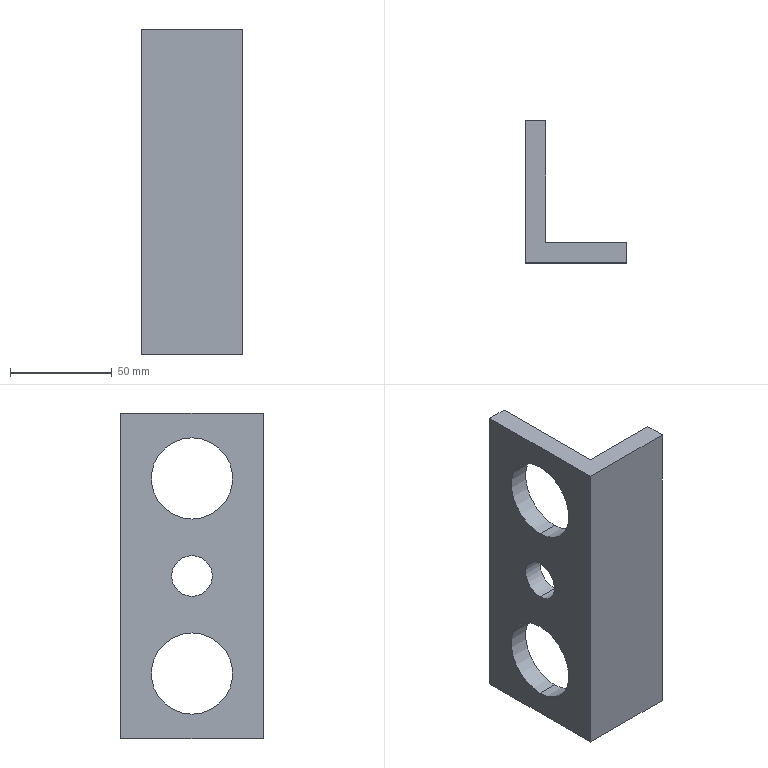Part | STEP file | 1 solid | 14 faces | box 50 x 70 x 160 mm | volume 147726 mm3 | plane 8 | cylinder 6 | commonest cylinder face diameters 40 x4 20 x2
STEP:
#1=CARTESIAN_POINT('',(0.,0.,0.));
#2=DIRECTION('',(0.,0.,1.));
#3=DIRECTION('',(1.,0.,0.));
#4=AXIS2_PLACEMENT_3D('',#1,#2,#3);
#5=CARTESIAN_POINT('',(-10.,25.,-10.));
#6=VERTEX_POINT('',#5);
#7=CARTESIAN_POINT('',(0.,25.,-10.));
#8=VERTEX_POINT('',#7);
#9=CARTESIAN_POINT('',(13.,25.,-10.));
#10=DIRECTION('',(1.,0.,0.));
#11=VECTOR('',#10,1.);
#12=LINE('',#9,#11);
#13=CARTESIAN_POINT('',(13.,25.,0.));
#14=DIRECTION('',(1.,0.,0.));
#15=DIRECTION('',(0.,0.,-1.));
#16=AXIS2_PLACEMENT_3D('',#13,#14,#15);
#17=CYLINDRICAL_SURFACE('',#16,10.);
#18=CARTESIAN_POINT('',(6.283,0.));
#19=DIRECTION('',(0.,1.));
#20=VECTOR('',#19,1.);
#21=LINE('',#18,#20);
#22=(GEOMETRIC_REPRESENTATION_CONTEXT(2)PARAMETRIC_REPRESENTATION_CONTEXT()REPRESENTATION_CONTEXT('',''));
#23=DEFINITIONAL_REPRESENTATION('',(#21),#22);
#24=PCURVE('',#17,#23);
#25=CARTESIAN_POINT('',(13.,25.,0.));
#26=DIRECTION('',(1.,0.,0.));
#27=DIRECTION('',(0.,0.,-1.));
#28=AXIS2_PLACEMENT_3D('',#25,#26,#27);
#29=CYLINDRICAL_SURFACE('',#28,10.);
#30=CARTESIAN_POINT('',(0.,0.));
#31=DIRECTION('',(0.,1.));
#32=VECTOR('',#31,1.);
#33=LINE('',#30,#32);
#34=(GEOMETRIC_REPRESENTATION_CONTEXT(2)PARAMETRIC_REPRESENTATION_CONTEXT()REPRESENTATION_CONTEXT('',''));
#35=DEFINITIONAL_REPRESENTATION('',(#33),#34);
#36=PCURVE('',#29,#35);
#37=SURFACE_CURVE('',#12,(#24,#36),.PCURVE_S1.);
#38=EDGE_CURVE('',#6,#8,#37,.T.);
#39=ORIENTED_EDGE('',*,*,#38,.T.);
#40=CARTESIAN_POINT('',(0.,25.,10.));
#41=VERTEX_POINT('',#40);
#42=CARTESIAN_POINT('',(0.,25.,0.));
#43=DIRECTION('',(-1.,0.,0.));
#44=DIRECTION('',(0.,0.,-1.));
#45=AXIS2_PLACEMENT_3D('',#42,#43,#44);
#46=CIRCLE('',#45,10.);
#47=CARTESIAN_POINT('',(6.283,-13.));
#48=DIRECTION('',(-1.,0.));
#49=VECTOR('',#48,1.);
#50=LINE('',#47,#49);
#51=(GEOMETRIC_REPRESENTATION_CONTEXT(2)PARAMETRIC_REPRESENTATION_CONTEXT()REPRESENTATION_CONTEXT('',''));
#52=DEFINITIONAL_REPRESENTATION('',(#50),#51);
#53=PCURVE('',#17,#52);
#54=CARTESIAN_POINT('',(0.,60.,80.));
#55=DIRECTION('',(1.,0.,0.));
#56=DIRECTION('',(0.,1.,0.));
#57=AXIS2_PLACEMENT_3D('',#54,#55,#56);
#58=PLANE('',#57);
#59=CARTESIAN_POINT('',(-35.,-90.));
#60=CARTESIAN_POINT('',(-52.321,-90.));
#61=CARTESIAN_POINT('',(-43.66,-75.));
#62=CARTESIAN_POINT('',(-35.,-60.));
#63=CARTESIAN_POINT('',(-26.34,-75.));
#64=CARTESIAN_POINT('',(-17.679,-90.));
#65=CARTESIAN_POINT('',(-35.,-90.));
#66=(BOUNDED_CURVE()B_SPLINE_CURVE(2,(#59,#60,#61,#62,#63,#64,#65),.UNSPECIFIED.,.T.,.F.)B_SPLINE_CURVE_WITH_KNOTS((1,2,2,2,2,1),(-2.094,0.,2.094,4.189,6.283,8.378),.UNSPECIFIED.)CURVE()GEOMETRIC_REPRESENTATION_ITEM()RATIONAL_B_SPLINE_CURVE((1.,0.5,1.,0.5,1.,0.5,1.))REPRESENTATION_ITEM(''));
#67=(GEOMETRIC_REPRESENTATION_CONTEXT(2)PARAMETRIC_REPRESENTATION_CONTEXT()REPRESENTATION_CONTEXT('',''));
#68=DEFINITIONAL_REPRESENTATION('',(#66),#67);
#69=PCURVE('',#58,#68);
#70=SURFACE_CURVE('',#46,(#53,#69),.PCURVE_S1.);
#71=EDGE_CURVE('',#8,#41,#70,.T.);
#72=ORIENTED_EDGE('',*,*,#71,.T.);
#73=CARTESIAN_POINT('',(-10.,25.,10.));
#74=VERTEX_POINT('',#73);
#75=CARTESIAN_POINT('',(13.,25.,10.));
#76=DIRECTION('',(1.,0.,0.));
#77=VECTOR('',#76,1.);
#78=LINE('',#75,#77);
#79=CARTESIAN_POINT('',(3.142,0.));
#80=DIRECTION('',(0.,1.));
#81=VECTOR('',#80,1.);
#82=LINE('',#79,#81);
#83=(GEOMETRIC_REPRESENTATION_CONTEXT(2)PARAMETRIC_REPRESENTATION_CONTEXT()REPRESENTATION_CONTEXT('',''));
#84=DEFINITIONAL_REPRESENTATION('',(#82),#83);
#85=PCURVE('',#17,#84);
#86=CARTESIAN_POINT('',(3.142,0.));
#87=DIRECTION('',(0.,1.));
#88=VECTOR('',#87,1.);
#89=LINE('',#86,#88);
#90=(GEOMETRIC_REPRESENTATION_CONTEXT(2)PARAMETRIC_REPRESENTATION_CONTEXT()REPRESENTATION_CONTEXT('',''));
#91=DEFINITIONAL_REPRESENTATION('',(#89),#90);
#92=PCURVE('',#29,#91);
#93=SURFACE_CURVE('',#78,(#85,#92),.PCURVE_S1.);
#94=EDGE_CURVE('',#74,#41,#93,.T.);
#95=ORIENTED_EDGE('',*,*,#94,.F.);
#96=CARTESIAN_POINT('',(-10.,25.,0.));
#97=DIRECTION('',(-1.,0.,0.));
#98=DIRECTION('',(0.,0.,-1.));
#99=AXIS2_PLACEMENT_3D('',#96,#97,#98);
#100=CIRCLE('',#99,10.);
#101=CARTESIAN_POINT('',(6.283,-23.));
#102=DIRECTION('',(-1.,0.));
#103=VECTOR('',#102,1.);
#104=LINE('',#101,#103);
#105=(GEOMETRIC_REPRESENTATION_CONTEXT(2)PARAMETRIC_REPRESENTATION_CONTEXT()REPRESENTATION_CONTEXT('',''));
#106=DEFINITIONAL_REPRESENTATION('',(#104),#105);
#107=PCURVE('',#17,#106);
#108=CARTESIAN_POINT('',(-10.,60.,80.));
#109=DIRECTION('',(1.,0.,0.));
#110=DIRECTION('',(0.,1.,0.));
#111=AXIS2_PLACEMENT_3D('',#108,#109,#110);
#112=PLANE('',#111);
#113=CARTESIAN_POINT('',(-35.,-90.));
#114=CARTESIAN_POINT('',(-52.321,-90.));
#115=CARTESIAN_POINT('',(-43.66,-75.));
#116=CARTESIAN_POINT('',(-35.,-60.));
#117=CARTESIAN_POINT('',(-26.34,-75.));
#118=CARTESIAN_POINT('',(-17.679,-90.));
#119=CARTESIAN_POINT('',(-35.,-90.));
#120=(BOUNDED_CURVE()B_SPLINE_CURVE(2,(#113,#114,#115,#116,#117,#118,#119),.UNSPECIFIED.,.T.,.F.)B_SPLINE_CURVE_WITH_KNOTS((1,2,2,2,2,1),(-2.094,0.,2.094,4.189,6.283,8.378),.UNSPECIFIED.)CURVE()GEOMETRIC_REPRESENTATION_ITEM()RATIONAL_B_SPLINE_CURVE((1.,0.5,1.,0.5,1.,0.5,1.))REPRESENTATION_ITEM(''));
#121=(GEOMETRIC_REPRESENTATION_CONTEXT(2)PARAMETRIC_REPRESENTATION_CONTEXT()REPRESENTATION_CONTEXT('',''));
#122=DEFINITIONAL_REPRESENTATION('',(#120),#121);
#123=PCURVE('',#112,#122);
#124=SURFACE_CURVE('',#100,(#107,#123),.PCURVE_S1.);
#125=EDGE_CURVE('',#6,#74,#124,.T.);
#126=ORIENTED_EDGE('',*,*,#125,.F.);
#127=EDGE_LOOP('',(#39,#72,#95,#126));
#128=FACE_BOUND('',#127,.F.);
#129=ADVANCED_FACE('',(#128),#17,.F.);
#130=CARTESIAN_POINT('',(-10.,25.,28.));
#131=VERTEX_POINT('',#130);
#132=CARTESIAN_POINT('',(0.,25.,28.));
#133=VERTEX_POINT('',#132);
#134=CARTESIAN_POINT('',(13.,25.,28.));
#135=DIRECTION('',(1.,0.,0.));
#136=VECTOR('',#135,1.);
#137=LINE('',#134,#136);
#138=CARTESIAN_POINT('',(13.,25.,48.));
#139=DIRECTION('',(1.,0.,0.));
#140=DIRECTION('',(0.,0.,-1.));
#141=AXIS2_PLACEMENT_3D('',#138,#139,#140);
#142=CYLINDRICAL_SURFACE('',#141,20.);
#143=CARTESIAN_POINT('',(6.283,0.));
#144=DIRECTION('',(0.,1.));
#145=VECTOR('',#144,1.);
#146=LINE('',#143,#145);
#147=(GEOMETRIC_REPRESENTATION_CONTEXT(2)PARAMETRIC_REPRESENTATION_CONTEXT()REPRESENTATION_CONTEXT('',''));
#148=DEFINITIONAL_REPRESENTATION('',(#146),#147);
#149=PCURVE('',#142,#148);
#150=CARTESIAN_POINT('',(13.,25.,48.));
#151=DIRECTION('',(1.,0.,0.));
#152=DIRECTION('',(0.,0.,-1.));
#153=AXIS2_PLACEMENT_3D('',#150,#151,#152);
#154=CYLINDRICAL_SURFACE('',#153,20.);
#155=CARTESIAN_POINT('',(0.,0.));
#156=DIRECTION('',(0.,1.));
#157=VECTOR('',#156,1.);
#158=LINE('',#155,#157);
#159=(GEOMETRIC_REPRESENTATION_CONTEXT(2)PARAMETRIC_REPRESENTATION_CONTEXT()REPRESENTATION_CONTEXT('',''));
#160=DEFINITIONAL_REPRESENTATION('',(#158),#159);
#161=PCURVE('',#154,#160);
#162=SURFACE_CURVE('',#137,(#149,#161),.PCURVE_S1.);
#163=EDGE_CURVE('',#131,#133,#162,.T.);
#164=ORIENTED_EDGE('',*,*,#163,.T.);
#165=CARTESIAN_POINT('',(0.,25.,68.));
#166=VERTEX_POINT('',#165);
#167=CARTESIAN_POINT('',(0.,25.,48.));
#168=DIRECTION('',(-1.,0.,0.));
#169=DIRECTION('',(0.,0.,-1.));
#170=AXIS2_PLACEMENT_3D('',#167,#168,#169);
#171=CIRCLE('',#170,20.);
#172=CARTESIAN_POINT('',(6.283,-13.));
#173=DIRECTION('',(-1.,0.));
#174=VECTOR('',#173,1.);
#175=LINE('',#172,#174);
#176=(GEOMETRIC_REPRESENTATION_CONTEXT(2)PARAMETRIC_REPRESENTATION_CONTEXT()REPRESENTATION_CONTEXT('',''));
#177=DEFINITIONAL_REPRESENTATION('',(#175),#176);
#178=PCURVE('',#142,#177);
#179=CARTESIAN_POINT('',(-35.,-52.));
#180=CARTESIAN_POINT('',(-69.641,-52.));
#181=CARTESIAN_POINT('',(-52.321,-22.));
#182=CARTESIAN_POINT('',(-35.,8.));
#183=CARTESIAN_POINT('',(-17.679,-22.));
#184=CARTESIAN_POINT('',(-0.359,-52.));
#185=CARTESIAN_POINT('',(-35.,-52.));
#186=(BOUNDED_CURVE()B_SPLINE_CURVE(2,(#179,#180,#181,#182,#183,#184,#185),.UNSPECIFIED.,.T.,.F.)B_SPLINE_CURVE_WITH_KNOTS((1,2,2,2,2,1),(-2.094,0.,2.094,4.189,6.283,8.378),.UNSPECIFIED.)CURVE()GEOMETRIC_REPRESENTATION_ITEM()RATIONAL_B_SPLINE_CURVE((1.,0.5,1.,0.5,1.,0.5,1.))REPRESENTATION_ITEM(''));
#187=(GEOMETRIC_REPRESENTATION_CONTEXT(2)PARAMETRIC_REPRESENTATION_CONTEXT()REPRESENTATION_CONTEXT('',''));
#188=DEFINITIONAL_REPRESENTATION('',(#186),#187);
#189=PCURVE('',#58,#188);
#190=SURFACE_CURVE('',#171,(#178,#189),.PCURVE_S1.);
#191=EDGE_CURVE('',#133,#166,#190,.T.);
#192=ORIENTED_EDGE('',*,*,#191,.T.);
#193=CARTESIAN_POINT('',(-10.,25.,68.));
#194=VERTEX_POINT('',#193);
#195=CARTESIAN_POINT('',(13.,25.,68.));
#196=DIRECTION('',(1.,0.,0.));
#197=VECTOR('',#196,1.);
#198=LINE('',#195,#197);
#199=CARTESIAN_POINT('',(3.142,0.));
#200=DIRECTION('',(0.,1.));
#201=VECTOR('',#200,1.);
#202=LINE('',#199,#201);
#203=(GEOMETRIC_REPRESENTATION_CONTEXT(2)PARAMETRIC_REPRESENTATION_CONTEXT()REPRESENTATION_CONTEXT('',''));
#204=DEFINITIONAL_REPRESENTATION('',(#202),#203);
#205=PCURVE('',#142,#204);
#206=CARTESIAN_POINT('',(3.142,0.));
#207=DIRECTION('',(0.,1.));
#208=VECTOR('',#207,1.);
#209=LINE('',#206,#208);
#210=(GEOMETRIC_REPRESENTATION_CONTEXT(2)PARAMETRIC_REPRESENTATION_CONTEXT()REPRESENTATION_CONTEXT('',''));
#211=DEFINITIONAL_REPRESENTATION('',(#209),#210);
#212=PCURVE('',#154,#211);
#213=SURFACE_CURVE('',#198,(#205,#212),.PCURVE_S1.);
#214=EDGE_CURVE('',#194,#166,#213,.T.);
#215=ORIENTED_EDGE('',*,*,#214,.F.);
#216=CARTESIAN_POINT('',(-10.,25.,48.));
#217=DIRECTION('',(-1.,0.,0.));
#218=DIRECTION('',(0.,0.,-1.));
#219=AXIS2_PLACEMENT_3D('',#216,#217,#218);
#220=CIRCLE('',#219,20.);
#221=CARTESIAN_POINT('',(6.283,-23.));
#222=DIRECTION('',(-1.,0.));
#223=VECTOR('',#222,1.);
#224=LINE('',#221,#223);
#225=(GEOMETRIC_REPRESENTATION_CONTEXT(2)PARAMETRIC_REPRESENTATION_CONTEXT()REPRESENTATION_CONTEXT('',''));
#226=DEFINITIONAL_REPRESENTATION('',(#224),#225);
#227=PCURVE('',#142,#226);
#228=CARTESIAN_POINT('',(-35.,-52.));
#229=CARTESIAN_POINT('',(-69.641,-52.));
#230=CARTESIAN_POINT('',(-52.321,-22.));
#231=CARTESIAN_POINT('',(-35.,8.));
#232=CARTESIAN_POINT('',(-17.679,-22.));
#233=CARTESIAN_POINT('',(-0.359,-52.));
#234=CARTESIAN_POINT('',(-35.,-52.));
#235=(BOUNDED_CURVE()B_SPLINE_CURVE(2,(#228,#229,#230,#231,#232,#233,#234),.UNSPECIFIED.,.T.,.F.)B_SPLINE_CURVE_WITH_KNOTS((1,2,2,2,2,1),(-2.094,0.,2.094,4.189,6.283,8.378),.UNSPECIFIED.)CURVE()GEOMETRIC_REPRESENTATION_ITEM()RATIONAL_B_SPLINE_CURVE((1.,0.5,1.,0.5,1.,0.5,1.))REPRESENTATION_ITEM(''));
#236=(GEOMETRIC_REPRESENTATION_CONTEXT(2)PARAMETRIC_REPRESENTATION_CONTEXT()REPRESENTATION_CONTEXT('',''));
#237=DEFINITIONAL_REPRESENTATION('',(#235),#236);
#238=PCURVE('',#112,#237);
#239=SURFACE_CURVE('',#220,(#227,#238),.PCURVE_S1.);
#240=EDGE_CURVE('',#131,#194,#239,.T.);
#241=ORIENTED_EDGE('',*,*,#240,.F.);
#242=EDGE_LOOP('',(#164,#192,#215,#241));
#243=FACE_BOUND('',#242,.F.);
#244=ADVANCED_FACE('',(#243),#142,.F.);
#245=CARTESIAN_POINT('',(-10.,25.,-68.));
#246=VERTEX_POINT('',#245);
#247=CARTESIAN_POINT('',(0.,25.,-68.));
#248=VERTEX_POINT('',#247);
#249=CARTESIAN_POINT('',(13.,25.,-68.));
#250=DIRECTION('',(1.,0.,0.));
#251=VECTOR('',#250,1.);
#252=LINE('',#249,#251);
#253=CARTESIAN_POINT('',(13.,25.,-48.));
#254=DIRECTION('',(1.,0.,0.));
#255=DIRECTION('',(0.,0.,-1.));
#256=AXIS2_PLACEMENT_3D('',#253,#254,#255);
#257=CYLINDRICAL_SURFACE('',#256,20.);
#258=CARTESIAN_POINT('',(6.283,0.));
#259=DIRECTION('',(0.,1.));
#260=VECTOR('',#259,1.);
#261=LINE('',#258,#260);
#262=(GEOMETRIC_REPRESENTATION_CONTEXT(2)PARAMETRIC_REPRESENTATION_CONTEXT()REPRESENTATION_CONTEXT('',''));
#263=DEFINITIONAL_REPRESENTATION('',(#261),#262);
#264=PCURVE('',#257,#263);
#265=CARTESIAN_POINT('',(13.,25.,-48.));
#266=DIRECTION('',(1.,0.,0.));
#267=DIRECTION('',(0.,0.,-1.));
#268=AXIS2_PLACEMENT_3D('',#265,#266,#267);
#269=CYLINDRICAL_SURFACE('',#268,20.);
#270=CARTESIAN_POINT('',(0.,0.));
#271=DIRECTION('',(0.,1.));
#272=VECTOR('',#271,1.);
#273=LINE('',#270,#272);
#274=(GEOMETRIC_REPRESENTATION_CONTEXT(2)PARAMETRIC_REPRESENTATION_CONTEXT()REPRESENTATION_CONTEXT('',''));
#275=DEFINITIONAL_REPRESENTATION('',(#273),#274);
#276=PCURVE('',#269,#275);
#277=SURFACE_CURVE('',#252,(#264,#276),.PCURVE_S1.);
#278=EDGE_CURVE('',#246,#248,#277,.T.);
#279=ORIENTED_EDGE('',*,*,#278,.T.);
#280=CARTESIAN_POINT('',(0.,25.,-28.));
#281=VERTEX_POINT('',#280);
#282=CARTESIAN_POINT('',(0.,25.,-48.));
#283=DIRECTION('',(-1.,0.,0.));
#284=DIRECTION('',(0.,0.,-1.));
#285=AXIS2_PLACEMENT_3D('',#282,#283,#284);
#286=CIRCLE('',#285,20.);
#287=CARTESIAN_POINT('',(6.283,-13.));
#288=DIRECTION('',(-1.,0.));
#289=VECTOR('',#288,1.);
#290=LINE('',#287,#289);
#291=(GEOMETRIC_REPRESENTATION_CONTEXT(2)PARAMETRIC_REPRESENTATION_CONTEXT()REPRESENTATION_CONTEXT('',''));
#292=DEFINITIONAL_REPRESENTATION('',(#290),#291);
#293=PCURVE('',#257,#292);
#294=CARTESIAN_POINT('',(-35.,-148.));
#295=CARTESIAN_POINT('',(-69.641,-148.));
#296=CARTESIAN_POINT('',(-52.321,-118.));
#297=CARTESIAN_POINT('',(-35.,-88.));
#298=CARTESIAN_POINT('',(-17.679,-118.));
#299=CARTESIAN_POINT('',(-0.359,-148.));
#300=CARTESIAN_POINT('',(-35.,-148.));
#301=(BOUNDED_CURVE()B_SPLINE_CURVE(2,(#294,#295,#296,#297,#298,#299,#300),.UNSPECIFIED.,.T.,.F.)B_SPLINE_CURVE_WITH_KNOTS((1,2,2,2,2,1),(-2.094,0.,2.094,4.189,6.283,8.378),.UNSPECIFIED.)CURVE()GEOMETRIC_REPRESENTATION_ITEM()RATIONAL_B_SPLINE_CURVE((1.,0.5,1.,0.5,1.,0.5,1.))REPRESENTATION_ITEM(''));
#302=(GEOMETRIC_REPRESENTATION_CONTEXT(2)PARAMETRIC_REPRESENTATION_CONTEXT()REPRESENTATION_CONTEXT('',''));
#303=DEFINITIONAL_REPRESENTATION('',(#301),#302);
#304=PCURVE('',#58,#303);
#305=SURFACE_CURVE('',#286,(#293,#304),.PCURVE_S1.);
#306=EDGE_CURVE('',#248,#281,#305,.T.);
#307=ORIENTED_EDGE('',*,*,#306,.T.);
#308=CARTESIAN_POINT('',(-10.,25.,-28.));
#309=VERTEX_POINT('',#308);
#310=CARTESIAN_POINT('',(13.,25.,-28.));
#311=DIRECTION('',(1.,0.,0.));
#312=VECTOR('',#311,1.);
#313=LINE('',#310,#312);
#314=CARTESIAN_POINT('',(3.142,0.));
#315=DIRECTION('',(0.,1.));
#316=VECTOR('',#315,1.);
#317=LINE('',#314,#316);
#318=(GEOMETRIC_REPRESENTATION_CONTEXT(2)PARAMETRIC_REPRESENTATION_CONTEXT()REPRESENTATION_CONTEXT('',''));
#319=DEFINITIONAL_REPRESENTATION('',(#317),#318);
#320=PCURVE('',#257,#319);
#321=CARTESIAN_POINT('',(3.142,0.));
#322=DIRECTION('',(0.,1.));
#323=VECTOR('',#322,1.);
#324=LINE('',#321,#323);
#325=(GEOMETRIC_REPRESENTATION_CONTEXT(2)PARAMETRIC_REPRESENTATION_CONTEXT()REPRESENTATION_CONTEXT('',''));
#326=DEFINITIONAL_REPRESENTATION('',(#324),#325);
#327=PCURVE('',#269,#326);
#328=SURFACE_CURVE('',#313,(#320,#327),.PCURVE_S1.);
#329=EDGE_CURVE('',#309,#281,#328,.T.);
#330=ORIENTED_EDGE('',*,*,#329,.F.);
#331=CARTESIAN_POINT('',(-10.,25.,-48.));
#332=DIRECTION('',(-1.,0.,0.));
#333=DIRECTION('',(0.,0.,-1.));
#334=AXIS2_PLACEMENT_3D('',#331,#332,#333);
#335=CIRCLE('',#334,20.);
#336=CARTESIAN_POINT('',(6.283,-23.));
#337=DIRECTION('',(-1.,0.));
#338=VECTOR('',#337,1.);
#339=LINE('',#336,#338);
#340=(GEOMETRIC_REPRESENTATION_CONTEXT(2)PARAMETRIC_REPRESENTATION_CONTEXT()REPRESENTATION_CONTEXT('',''));
#341=DEFINITIONAL_REPRESENTATION('',(#339),#340);
#342=PCURVE('',#257,#341);
#343=CARTESIAN_POINT('',(-35.,-148.));
#344=CARTESIAN_POINT('',(-69.641,-148.));
#345=CARTESIAN_POINT('',(-52.321,-118.));
#346=CARTESIAN_POINT('',(-35.,-88.));
#347=CARTESIAN_POINT('',(-17.679,-118.));
#348=CARTESIAN_POINT('',(-0.359,-148.));
#349=CARTESIAN_POINT('',(-35.,-148.));
#350=(BOUNDED_CURVE()B_SPLINE_CURVE(2,(#343,#344,#345,#346,#347,#348,#349),.UNSPECIFIED.,.T.,.F.)B_SPLINE_CURVE_WITH_KNOTS((1,2,2,2,2,1),(-2.094,0.,2.094,4.189,6.283,8.378),.UNSPECIFIED.)CURVE()GEOMETRIC_REPRESENTATION_ITEM()RATIONAL_B_SPLINE_CURVE((1.,0.5,1.,0.5,1.,0.5,1.))REPRESENTATION_ITEM(''));
#351=(GEOMETRIC_REPRESENTATION_CONTEXT(2)PARAMETRIC_REPRESENTATION_CONTEXT()REPRESENTATION_CONTEXT('',''));
#352=DEFINITIONAL_REPRESENTATION('',(#350),#351);
#353=PCURVE('',#112,#352);
#354=SURFACE_CURVE('',#335,(#342,#353),.PCURVE_S1.);
#355=EDGE_CURVE('',#246,#309,#354,.T.);
#356=ORIENTED_EDGE('',*,*,#355,.F.);
#357=EDGE_LOOP('',(#279,#307,#330,#356));
#358=FACE_BOUND('',#357,.F.);
#359=ADVANCED_FACE('',(#358),#257,.F.);
#360=ORIENTED_EDGE('',*,*,#125,.F.);
#361=CARTESIAN_POINT('',(-10.,25.,0.));
#362=DIRECTION('',(-1.,0.,0.));
#363=DIRECTION('',(0.,0.,-1.));
#364=AXIS2_PLACEMENT_3D('',#361,#362,#363);
#365=CIRCLE('',#364,10.);
#366=CARTESIAN_POINT('',(-35.,-90.));
#367=CARTESIAN_POINT('',(-52.321,-90.));
#368=CARTESIAN_POINT('',(-43.66,-75.));
#369=CARTESIAN_POINT('',(-35.,-60.));
#370=CARTESIAN_POINT('',(-26.34,-75.));
#371=CARTESIAN_POINT('',(-17.679,-90.));
#372=CARTESIAN_POINT('',(-35.,-90.));
#373=(BOUNDED_CURVE()B_SPLINE_CURVE(2,(#366,#367,#368,#369,#370,#371,#372),.UNSPECIFIED.,.T.,.F.)B_SPLINE_CURVE_WITH_KNOTS((1,2,2,2,2,1),(-2.094,0.,2.094,4.189,6.283,8.378),.UNSPECIFIED.)CURVE()GEOMETRIC_REPRESENTATION_ITEM()RATIONAL_B_SPLINE_CURVE((1.,0.5,1.,0.5,1.,0.5,1.))REPRESENTATION_ITEM(''));
#374=(GEOMETRIC_REPRESENTATION_CONTEXT(2)PARAMETRIC_REPRESENTATION_CONTEXT()REPRESENTATION_CONTEXT('',''));
#375=DEFINITIONAL_REPRESENTATION('',(#373),#374);
#376=PCURVE('',#112,#375);
#377=CARTESIAN_POINT('',(6.283,-23.));
#378=DIRECTION('',(-1.,0.));
#379=VECTOR('',#378,1.);
#380=LINE('',#377,#379);
#381=(GEOMETRIC_REPRESENTATION_CONTEXT(2)PARAMETRIC_REPRESENTATION_CONTEXT()REPRESENTATION_CONTEXT('',''));
#382=DEFINITIONAL_REPRESENTATION('',(#380),#381);
#383=PCURVE('',#29,#382);
#384=SURFACE_CURVE('',#365,(#376,#383),.PCURVE_S1.);
#385=EDGE_CURVE('',#74,#6,#384,.T.);
#386=ORIENTED_EDGE('',*,*,#385,.F.);
#387=EDGE_LOOP('',(#360,#386));
#388=FACE_BOUND('',#387,.T.);
#389=ORIENTED_EDGE('',*,*,#240,.F.);
#390=CARTESIAN_POINT('',(-10.,25.,48.));
#391=DIRECTION('',(-1.,0.,0.));
#392=DIRECTION('',(0.,0.,-1.));
#393=AXIS2_PLACEMENT_3D('',#390,#391,#392);
#394=CIRCLE('',#393,20.);
#395=CARTESIAN_POINT('',(-35.,-52.));
#396=CARTESIAN_POINT('',(-69.641,-52.));
#397=CARTESIAN_POINT('',(-52.321,-22.));
#398=CARTESIAN_POINT('',(-35.,8.));
#399=CARTESIAN_POINT('',(-17.679,-22.));
#400=CARTESIAN_POINT('',(-0.359,-52.));
#401=CARTESIAN_POINT('',(-35.,-52.));
#402=(BOUNDED_CURVE()B_SPLINE_CURVE(2,(#395,#396,#397,#398,#399,#400,#401),.UNSPECIFIED.,.T.,.F.)B_SPLINE_CURVE_WITH_KNOTS((1,2,2,2,2,1),(-2.094,0.,2.094,4.189,6.283,8.378),.UNSPECIFIED.)CURVE()GEOMETRIC_REPRESENTATION_ITEM()RATIONAL_B_SPLINE_CURVE((1.,0.5,1.,0.5,1.,0.5,1.))REPRESENTATION_ITEM(''));
#403=(GEOMETRIC_REPRESENTATION_CONTEXT(2)PARAMETRIC_REPRESENTATION_CONTEXT()REPRESENTATION_CONTEXT('',''));
#404=DEFINITIONAL_REPRESENTATION('',(#402),#403);
#405=PCURVE('',#112,#404);
#406=CARTESIAN_POINT('',(6.283,-23.));
#407=DIRECTION('',(-1.,0.));
#408=VECTOR('',#407,1.);
#409=LINE('',#406,#408);
#410=(GEOMETRIC_REPRESENTATION_CONTEXT(2)PARAMETRIC_REPRESENTATION_CONTEXT()REPRESENTATION_CONTEXT('',''));
#411=DEFINITIONAL_REPRESENTATION('',(#409),#410);
#412=PCURVE('',#154,#411);
#413=SURFACE_CURVE('',#394,(#405,#412),.PCURVE_S1.);
#414=EDGE_CURVE('',#194,#131,#413,.T.);
#415=ORIENTED_EDGE('',*,*,#414,.F.);
#416=EDGE_LOOP('',(#389,#415));
#417=FACE_BOUND('',#416,.T.);
#418=ORIENTED_EDGE('',*,*,#355,.F.);
#419=CARTESIAN_POINT('',(-10.,25.,-48.));
#420=DIRECTION('',(-1.,0.,0.));
#421=DIRECTION('',(0.,0.,-1.));
#422=AXIS2_PLACEMENT_3D('',#419,#420,#421);
#423=CIRCLE('',#422,20.);
#424=CARTESIAN_POINT('',(-35.,-148.));
#425=CARTESIAN_POINT('',(-69.641,-148.));
#426=CARTESIAN_POINT('',(-52.321,-118.));
#427=CARTESIAN_POINT('',(-35.,-88.));
#428=CARTESIAN_POINT('',(-17.679,-118.));
#429=CARTESIAN_POINT('',(-0.359,-148.));
#430=CARTESIAN_POINT('',(-35.,-148.));
#431=(BOUNDED_CURVE()B_SPLINE_CURVE(2,(#424,#425,#426,#427,#428,#429,#430),.UNSPECIFIED.,.T.,.F.)B_SPLINE_CURVE_WITH_KNOTS((1,2,2,2,2,1),(-2.094,0.,2.094,4.189,6.283,8.378),.UNSPECIFIED.)CURVE()GEOMETRIC_REPRESENTATION_ITEM()RATIONAL_B_SPLINE_CURVE((1.,0.5,1.,0.5,1.,0.5,1.))REPRESENTATION_ITEM(''));
#432=(GEOMETRIC_REPRESENTATION_CONTEXT(2)PARAMETRIC_REPRESENTATION_CONTEXT()REPRESENTATION_CONTEXT('',''));
#433=DEFINITIONAL_REPRESENTATION('',(#431),#432);
#434=PCURVE('',#112,#433);
#435=CARTESIAN_POINT('',(6.283,-23.));
#436=DIRECTION('',(-1.,0.));
#437=VECTOR('',#436,1.);
#438=LINE('',#435,#437);
#439=(GEOMETRIC_REPRESENTATION_CONTEXT(2)PARAMETRIC_REPRESENTATION_CONTEXT()REPRESENTATION_CONTEXT('',''));
#440=DEFINITIONAL_REPRESENTATION('',(#438),#439);
#441=PCURVE('',#269,#440);
#442=SURFACE_CURVE('',#423,(#434,#441),.PCURVE_S1.);
#443=EDGE_CURVE('',#309,#246,#442,.T.);
#444=ORIENTED_EDGE('',*,*,#443,.F.);
#445=EDGE_LOOP('',(#418,#444));
#446=FACE_BOUND('',#445,.T.);
#447=CARTESIAN_POINT('',(-10.,-10.,80.));
#448=VERTEX_POINT('',#447);
#449=CARTESIAN_POINT('',(-10.,-10.,-80.));
#450=VERTEX_POINT('',#449);
#451=CARTESIAN_POINT('',(-10.,-10.,80.));
#452=DIRECTION('',(0.,0.,-1.));
#453=VECTOR('',#452,1.);
#454=LINE('',#451,#453);
#455=CARTESIAN_POINT('',(-70.,0.));
#456=DIRECTION('',(0.,-1.));
#457=VECTOR('',#456,1.);
#458=LINE('',#455,#457);
#459=(GEOMETRIC_REPRESENTATION_CONTEXT(2)PARAMETRIC_REPRESENTATION_CONTEXT()REPRESENTATION_CONTEXT('',''));
#460=DEFINITIONAL_REPRESENTATION('',(#458),#459);
#461=PCURVE('',#112,#460);
#462=CARTESIAN_POINT('',(0.,-10.,80.));
#463=DIRECTION('',(0.,1.,0.));
#464=DIRECTION('',(0.,0.,1.));
#465=AXIS2_PLACEMENT_3D('',#462,#463,#464);
#466=PLANE('',#465);
#467=CARTESIAN_POINT('',(0.,-10.));
#468=DIRECTION('',(-1.,0.));
#469=VECTOR('',#468,1.);
#470=LINE('',#467,#469);
#471=(GEOMETRIC_REPRESENTATION_CONTEXT(2)PARAMETRIC_REPRESENTATION_CONTEXT()REPRESENTATION_CONTEXT('',''));
#472=DEFINITIONAL_REPRESENTATION('',(#470),#471);
#473=PCURVE('',#466,#472);
#474=SURFACE_CURVE('',#454,(#461,#473),.PCURVE_S1.);
#475=EDGE_CURVE('',#448,#450,#474,.T.);
#476=ORIENTED_EDGE('',*,*,#475,.F.);
#477=CARTESIAN_POINT('',(-10.,60.,80.));
#478=VERTEX_POINT('',#477);
#479=CARTESIAN_POINT('',(-10.,60.,80.));
#480=DIRECTION('',(0.,-1.,0.));
#481=VECTOR('',#480,1.);
#482=LINE('',#479,#481);
#483=CARTESIAN_POINT('',(0.,0.));
#484=DIRECTION('',(-1.,0.));
#485=VECTOR('',#484,1.);
#486=LINE('',#483,#485);
#487=(GEOMETRIC_REPRESENTATION_CONTEXT(2)PARAMETRIC_REPRESENTATION_CONTEXT()REPRESENTATION_CONTEXT('',''));
#488=DEFINITIONAL_REPRESENTATION('',(#486),#487);
#489=PCURVE('',#112,#488);
#490=CARTESIAN_POINT('',(0.,0.,80.));
#491=DIRECTION('',(0.,0.,-1.));
#492=DIRECTION('',(-1.,0.,0.));
#493=AXIS2_PLACEMENT_3D('',#490,#491,#492);
#494=PLANE('',#493);
#495=CARTESIAN_POINT('',(10.,60.));
#496=DIRECTION('',(0.,-1.));
#497=VECTOR('',#496,1.);
#498=LINE('',#495,#497);
#499=(GEOMETRIC_REPRESENTATION_CONTEXT(2)PARAMETRIC_REPRESENTATION_CONTEXT()REPRESENTATION_CONTEXT('',''));
#500=DEFINITIONAL_REPRESENTATION('',(#498),#499);
#501=PCURVE('',#494,#500);
#502=SURFACE_CURVE('',#482,(#489,#501),.PCURVE_S1.);
#503=EDGE_CURVE('',#478,#448,#502,.T.);
#504=ORIENTED_EDGE('',*,*,#503,.F.);
#505=CARTESIAN_POINT('',(-10.,60.,-80.));
#506=VERTEX_POINT('',#505);
#507=CARTESIAN_POINT('',(-10.,60.,80.));
#508=DIRECTION('',(0.,0.,1.));
#509=VECTOR('',#508,1.);
#510=LINE('',#507,#509);
#511=CARTESIAN_POINT('',(0.,0.));
#512=DIRECTION('',(0.,1.));
#513=VECTOR('',#512,1.);
#514=LINE('',#511,#513);
#515=(GEOMETRIC_REPRESENTATION_CONTEXT(2)PARAMETRIC_REPRESENTATION_CONTEXT()REPRESENTATION_CONTEXT('',''));
#516=DEFINITIONAL_REPRESENTATION('',(#514),#515);
#517=PCURVE('',#112,#516);
#518=CARTESIAN_POINT('',(-10.,60.,80.));
#519=DIRECTION('',(0.,1.,0.));
#520=DIRECTION('',(0.,0.,1.));
#521=AXIS2_PLACEMENT_3D('',#518,#519,#520);
#522=PLANE('',#521);
#523=CARTESIAN_POINT('',(0.,0.));
#524=DIRECTION('',(1.,0.));
#525=VECTOR('',#524,1.);
#526=LINE('',#523,#525);
#527=(GEOMETRIC_REPRESENTATION_CONTEXT(2)PARAMETRIC_REPRESENTATION_CONTEXT()REPRESENTATION_CONTEXT('',''));
#528=DEFINITIONAL_REPRESENTATION('',(#526),#527);
#529=PCURVE('',#522,#528);
#530=SURFACE_CURVE('',#510,(#517,#529),.PCURVE_S1.);
#531=EDGE_CURVE('',#506,#478,#530,.T.);
#532=ORIENTED_EDGE('',*,*,#531,.F.);
#533=CARTESIAN_POINT('',(-10.,60.,-80.));
#534=DIRECTION('',(0.,1.,0.));
#535=VECTOR('',#534,1.);
#536=LINE('',#533,#535);
#537=CARTESIAN_POINT('',(0.,-160.));
#538=DIRECTION('',(1.,0.));
#539=VECTOR('',#538,1.);
#540=LINE('',#537,#539);
#541=(GEOMETRIC_REPRESENTATION_CONTEXT(2)PARAMETRIC_REPRESENTATION_CONTEXT()REPRESENTATION_CONTEXT('',''));
#542=DEFINITIONAL_REPRESENTATION('',(#540),#541);
#543=PCURVE('',#112,#542);
#544=CARTESIAN_POINT('',(0.,0.,-80.));
#545=DIRECTION('',(0.,0.,-1.));
#546=DIRECTION('',(-1.,0.,0.));
#547=AXIS2_PLACEMENT_3D('',#544,#545,#546);
#548=PLANE('',#547);
#549=CARTESIAN_POINT('',(10.,60.));
#550=DIRECTION('',(0.,1.));
#551=VECTOR('',#550,1.);
#552=LINE('',#549,#551);
#553=(GEOMETRIC_REPRESENTATION_CONTEXT(2)PARAMETRIC_REPRESENTATION_CONTEXT()REPRESENTATION_CONTEXT('',''));
#554=DEFINITIONAL_REPRESENTATION('',(#552),#553);
#555=PCURVE('',#548,#554);
#556=SURFACE_CURVE('',#536,(#543,#555),.PCURVE_S1.);
#557=EDGE_CURVE('',#450,#506,#556,.T.);
#558=ORIENTED_EDGE('',*,*,#557,.F.);
#559=EDGE_LOOP('',(#476,#504,#532,#558));
#560=FACE_BOUND('',#559,.T.);
#561=ADVANCED_FACE('',(#388,#417,#446,#560),#112,.F.);
#562=CARTESIAN_POINT('',(0.,25.,0.));
#563=DIRECTION('',(-1.,0.,0.));
#564=DIRECTION('',(0.,0.,-1.));
#565=AXIS2_PLACEMENT_3D('',#562,#563,#564);
#566=CIRCLE('',#565,10.);
#567=CARTESIAN_POINT('',(6.283,-13.));
#568=DIRECTION('',(-1.,0.));
#569=VECTOR('',#568,1.);
#570=LINE('',#567,#569);
#571=(GEOMETRIC_REPRESENTATION_CONTEXT(2)PARAMETRIC_REPRESENTATION_CONTEXT()REPRESENTATION_CONTEXT('',''));
#572=DEFINITIONAL_REPRESENTATION('',(#570),#571);
#573=PCURVE('',#29,#572);
#574=CARTESIAN_POINT('',(-35.,-90.));
#575=CARTESIAN_POINT('',(-52.321,-90.));
#576=CARTESIAN_POINT('',(-43.66,-75.));
#577=CARTESIAN_POINT('',(-35.,-60.));
#578=CARTESIAN_POINT('',(-26.34,-75.));
#579=CARTESIAN_POINT('',(-17.679,-90.));
#580=CARTESIAN_POINT('',(-35.,-90.));
#581=(BOUNDED_CURVE()B_SPLINE_CURVE(2,(#574,#575,#576,#577,#578,#579,#580),.UNSPECIFIED.,.T.,.F.)B_SPLINE_CURVE_WITH_KNOTS((1,2,2,2,2,1),(-2.094,0.,2.094,4.189,6.283,8.378),.UNSPECIFIED.)CURVE()GEOMETRIC_REPRESENTATION_ITEM()RATIONAL_B_SPLINE_CURVE((1.,0.5,1.,0.5,1.,0.5,1.))REPRESENTATION_ITEM(''));
#582=(GEOMETRIC_REPRESENTATION_CONTEXT(2)PARAMETRIC_REPRESENTATION_CONTEXT()REPRESENTATION_CONTEXT('',''));
#583=DEFINITIONAL_REPRESENTATION('',(#581),#582);
#584=PCURVE('',#58,#583);
#585=SURFACE_CURVE('',#566,(#573,#584),.PCURVE_S1.);
#586=EDGE_CURVE('',#41,#8,#585,.T.);
#587=ORIENTED_EDGE('',*,*,#586,.T.);
#588=ORIENTED_EDGE('',*,*,#38,.F.);
#589=ORIENTED_EDGE('',*,*,#385,.F.);
#590=ORIENTED_EDGE('',*,*,#94,.T.);
#591=EDGE_LOOP('',(#587,#588,#589,#590));
#592=FACE_BOUND('',#591,.F.);
#593=ADVANCED_FACE('',(#592),#29,.F.);
#594=CARTESIAN_POINT('',(0.,25.,48.));
#595=DIRECTION('',(-1.,0.,0.));
#596=DIRECTION('',(0.,0.,-1.));
#597=AXIS2_PLACEMENT_3D('',#594,#595,#596);
#598=CIRCLE('',#597,20.);
#599=CARTESIAN_POINT('',(6.283,-13.));
#600=DIRECTION('',(-1.,0.));
#601=VECTOR('',#600,1.);
#602=LINE('',#599,#601);
#603=(GEOMETRIC_REPRESENTATION_CONTEXT(2)PARAMETRIC_REPRESENTATION_CONTEXT()REPRESENTATION_CONTEXT('',''));
#604=DEFINITIONAL_REPRESENTATION('',(#602),#603);
#605=PCURVE('',#154,#604);
#606=CARTESIAN_POINT('',(-35.,-52.));
#607=CARTESIAN_POINT('',(-69.641,-52.));
#608=CARTESIAN_POINT('',(-52.321,-22.));
#609=CARTESIAN_POINT('',(-35.,8.));
#610=CARTESIAN_POINT('',(-17.679,-22.));
#611=CARTESIAN_POINT('',(-0.359,-52.));
#612=CARTESIAN_POINT('',(-35.,-52.));
#613=(BOUNDED_CURVE()B_SPLINE_CURVE(2,(#606,#607,#608,#609,#610,#611,#612),.UNSPECIFIED.,.T.,.F.)B_SPLINE_CURVE_WITH_KNOTS((1,2,2,2,2,1),(-2.094,0.,2.094,4.189,6.283,8.378),.UNSPECIFIED.)CURVE()GEOMETRIC_REPRESENTATION_ITEM()RATIONAL_B_SPLINE_CURVE((1.,0.5,1.,0.5,1.,0.5,1.))REPRESENTATION_ITEM(''));
#614=(GEOMETRIC_REPRESENTATION_CONTEXT(2)PARAMETRIC_REPRESENTATION_CONTEXT()REPRESENTATION_CONTEXT('',''));
#615=DEFINITIONAL_REPRESENTATION('',(#613),#614);
#616=PCURVE('',#58,#615);
#617=SURFACE_CURVE('',#598,(#605,#616),.PCURVE_S1.);
#618=EDGE_CURVE('',#166,#133,#617,.T.);
#619=ORIENTED_EDGE('',*,*,#618,.T.);
#620=ORIENTED_EDGE('',*,*,#163,.F.);
#621=ORIENTED_EDGE('',*,*,#414,.F.);
#622=ORIENTED_EDGE('',*,*,#214,.T.);
#623=EDGE_LOOP('',(#619,#620,#621,#622));
#624=FACE_BOUND('',#623,.F.);
#625=ADVANCED_FACE('',(#624),#154,.F.);
#626=CARTESIAN_POINT('',(0.,25.,-48.));
#627=DIRECTION('',(-1.,0.,0.));
#628=DIRECTION('',(0.,0.,-1.));
#629=AXIS2_PLACEMENT_3D('',#626,#627,#628);
#630=CIRCLE('',#629,20.);
#631=CARTESIAN_POINT('',(6.283,-13.));
#632=DIRECTION('',(-1.,0.));
#633=VECTOR('',#632,1.);
#634=LINE('',#631,#633);
#635=(GEOMETRIC_REPRESENTATION_CONTEXT(2)PARAMETRIC_REPRESENTATION_CONTEXT()REPRESENTATION_CONTEXT('',''));
#636=DEFINITIONAL_REPRESENTATION('',(#634),#635);
#637=PCURVE('',#269,#636);
#638=CARTESIAN_POINT('',(-35.,-148.));
#639=CARTESIAN_POINT('',(-69.641,-148.));
#640=CARTESIAN_POINT('',(-52.321,-118.));
#641=CARTESIAN_POINT('',(-35.,-88.));
#642=CARTESIAN_POINT('',(-17.679,-118.));
#643=CARTESIAN_POINT('',(-0.359,-148.));
#644=CARTESIAN_POINT('',(-35.,-148.));
#645=(BOUNDED_CURVE()B_SPLINE_CURVE(2,(#638,#639,#640,#641,#642,#643,#644),.UNSPECIFIED.,.T.,.F.)B_SPLINE_CURVE_WITH_KNOTS((1,2,2,2,2,1),(-2.094,0.,2.094,4.189,6.283,8.378),.UNSPECIFIED.)CURVE()GEOMETRIC_REPRESENTATION_ITEM()RATIONAL_B_SPLINE_CURVE((1.,0.5,1.,0.5,1.,0.5,1.))REPRESENTATION_ITEM(''));
#646=(GEOMETRIC_REPRESENTATION_CONTEXT(2)PARAMETRIC_REPRESENTATION_CONTEXT()REPRESENTATION_CONTEXT('',''));
#647=DEFINITIONAL_REPRESENTATION('',(#645),#646);
#648=PCURVE('',#58,#647);
#649=SURFACE_CURVE('',#630,(#637,#648),.PCURVE_S1.);
#650=EDGE_CURVE('',#281,#248,#649,.T.);
#651=ORIENTED_EDGE('',*,*,#650,.T.);
#652=ORIENTED_EDGE('',*,*,#278,.F.);
#653=ORIENTED_EDGE('',*,*,#443,.F.);
#654=ORIENTED_EDGE('',*,*,#329,.T.);
#655=EDGE_LOOP('',(#651,#652,#653,#654));
#656=FACE_BOUND('',#655,.F.);
#657=ADVANCED_FACE('',(#656),#269,.F.);
#658=CARTESIAN_POINT('',(0.,0.,-80.));
#659=VERTEX_POINT('',#658);
#660=CARTESIAN_POINT('',(40.,0.,-80.));
#661=VERTEX_POINT('',#660);
#662=CARTESIAN_POINT('',(0.,0.,-80.));
#663=DIRECTION('',(1.,0.,0.));
#664=VECTOR('',#663,1.);
#665=LINE('',#662,#664);
#666=CARTESIAN_POINT('',(0.,0.));
#667=DIRECTION('',(-1.,0.));
#668=VECTOR('',#667,1.);
#669=LINE('',#666,#668);
#670=(GEOMETRIC_REPRESENTATION_CONTEXT(2)PARAMETRIC_REPRESENTATION_CONTEXT()REPRESENTATION_CONTEXT('',''));
#671=DEFINITIONAL_REPRESENTATION('',(#669),#670);
#672=PCURVE('',#548,#671);
#673=CARTESIAN_POINT('',(0.,0.,80.));
#674=DIRECTION('',(0.,1.,0.));
#675=DIRECTION('',(0.,0.,1.));
#676=AXIS2_PLACEMENT_3D('',#673,#674,#675);
#677=PLANE('',#676);
#678=CARTESIAN_POINT('',(-160.,0.));
#679=DIRECTION('',(0.,1.));
#680=VECTOR('',#679,1.);
#681=LINE('',#678,#680);
#682=(GEOMETRIC_REPRESENTATION_CONTEXT(2)PARAMETRIC_REPRESENTATION_CONTEXT()REPRESENTATION_CONTEXT('',''));
#683=DEFINITIONAL_REPRESENTATION('',(#681),#682);
#684=PCURVE('',#677,#683);
#685=SURFACE_CURVE('',#665,(#672,#684),.PCURVE_S1.);
#686=EDGE_CURVE('',#659,#661,#685,.T.);
#687=ORIENTED_EDGE('',*,*,#686,.T.);
#688=CARTESIAN_POINT('',(40.,-10.,-80.));
#689=VERTEX_POINT('',#688);
#690=CARTESIAN_POINT('',(40.,0.,-80.));
#691=DIRECTION('',(0.,-1.,0.));
#692=VECTOR('',#691,1.);
#693=LINE('',#690,#692);
#694=CARTESIAN_POINT('',(-40.,0.));
#695=DIRECTION('',(0.,-1.));
#696=VECTOR('',#695,1.);
#697=LINE('',#694,#696);
#698=(GEOMETRIC_REPRESENTATION_CONTEXT(2)PARAMETRIC_REPRESENTATION_CONTEXT()REPRESENTATION_CONTEXT('',''));
#699=DEFINITIONAL_REPRESENTATION('',(#697),#698);
#700=PCURVE('',#548,#699);
#701=CARTESIAN_POINT('',(40.,0.,80.));
#702=DIRECTION('',(1.,0.,0.));
#703=DIRECTION('',(0.,0.,-1.));
#704=AXIS2_PLACEMENT_3D('',#701,#702,#703);
#705=PLANE('',#704);
#706=CARTESIAN_POINT('',(160.,0.));
#707=DIRECTION('',(0.,-1.));
#708=VECTOR('',#707,1.);
#709=LINE('',#706,#708);
#710=(GEOMETRIC_REPRESENTATION_CONTEXT(2)PARAMETRIC_REPRESENTATION_CONTEXT()REPRESENTATION_CONTEXT('',''));
#711=DEFINITIONAL_REPRESENTATION('',(#709),#710);
#712=PCURVE('',#705,#711);
#713=SURFACE_CURVE('',#693,(#700,#712),.PCURVE_S1.);
#714=EDGE_CURVE('',#661,#689,#713,.T.);
#715=ORIENTED_EDGE('',*,*,#714,.T.);
#716=CARTESIAN_POINT('',(0.,-10.,-80.));
#717=DIRECTION('',(-1.,0.,0.));
#718=VECTOR('',#717,1.);
#719=LINE('',#716,#718);
#720=CARTESIAN_POINT('',(0.,-10.));
#721=DIRECTION('',(1.,0.));
#722=VECTOR('',#721,1.);
#723=LINE('',#720,#722);
#724=(GEOMETRIC_REPRESENTATION_CONTEXT(2)PARAMETRIC_REPRESENTATION_CONTEXT()REPRESENTATION_CONTEXT('',''));
#725=DEFINITIONAL_REPRESENTATION('',(#723),#724);
#726=PCURVE('',#548,#725);
#727=CARTESIAN_POINT('',(-160.,0.));
#728=DIRECTION('',(0.,-1.));
#729=VECTOR('',#728,1.);
#730=LINE('',#727,#729);
#731=(GEOMETRIC_REPRESENTATION_CONTEXT(2)PARAMETRIC_REPRESENTATION_CONTEXT()REPRESENTATION_CONTEXT('',''));
#732=DEFINITIONAL_REPRESENTATION('',(#730),#731);
#733=PCURVE('',#466,#732);
#734=SURFACE_CURVE('',#719,(#726,#733),.PCURVE_S1.);
#735=EDGE_CURVE('',#689,#450,#734,.T.);
#736=ORIENTED_EDGE('',*,*,#735,.T.);
#737=ORIENTED_EDGE('',*,*,#557,.T.);
#738=CARTESIAN_POINT('',(0.,60.,-80.));
#739=VERTEX_POINT('',#738);
#740=CARTESIAN_POINT('',(0.,60.,-80.));
#741=DIRECTION('',(1.,0.,0.));
#742=VECTOR('',#741,1.);
#743=LINE('',#740,#742);
#744=CARTESIAN_POINT('',(0.,60.));
#745=DIRECTION('',(-1.,0.));
#746=VECTOR('',#745,1.);
#747=LINE('',#744,#746);
#748=(GEOMETRIC_REPRESENTATION_CONTEXT(2)PARAMETRIC_REPRESENTATION_CONTEXT()REPRESENTATION_CONTEXT('',''));
#749=DEFINITIONAL_REPRESENTATION('',(#747),#748);
#750=PCURVE('',#548,#749);
#751=CARTESIAN_POINT('',(-160.,10.));
#752=DIRECTION('',(0.,1.));
#753=VECTOR('',#752,1.);
#754=LINE('',#751,#753);
#755=(GEOMETRIC_REPRESENTATION_CONTEXT(2)PARAMETRIC_REPRESENTATION_CONTEXT()REPRESENTATION_CONTEXT('',''));
#756=DEFINITIONAL_REPRESENTATION('',(#754),#755);
#757=PCURVE('',#522,#756);
#758=SURFACE_CURVE('',#743,(#750,#757),.PCURVE_S1.);
#759=EDGE_CURVE('',#506,#739,#758,.T.);
#760=ORIENTED_EDGE('',*,*,#759,.T.);
#761=CARTESIAN_POINT('',(0.,0.,-80.));
#762=DIRECTION('',(0.,-1.,0.));
#763=VECTOR('',#762,1.);
#764=LINE('',#761,#763);
#765=CARTESIAN_POINT('',(0.,0.));
#766=DIRECTION('',(0.,-1.));
#767=VECTOR('',#766,1.);
#768=LINE('',#765,#767);
#769=(GEOMETRIC_REPRESENTATION_CONTEXT(2)PARAMETRIC_REPRESENTATION_CONTEXT()REPRESENTATION_CONTEXT('',''));
#770=DEFINITIONAL_REPRESENTATION('',(#768),#769);
#771=PCURVE('',#548,#770);
#772=CARTESIAN_POINT('',(-60.,-160.));
#773=DIRECTION('',(-1.,0.));
#774=VECTOR('',#773,1.);
#775=LINE('',#772,#774);
#776=(GEOMETRIC_REPRESENTATION_CONTEXT(2)PARAMETRIC_REPRESENTATION_CONTEXT()REPRESENTATION_CONTEXT('',''));
#777=DEFINITIONAL_REPRESENTATION('',(#775),#776);
#778=PCURVE('',#58,#777);
#779=SURFACE_CURVE('',#764,(#771,#778),.PCURVE_S1.);
#780=EDGE_CURVE('',#739,#659,#779,.T.);
#781=ORIENTED_EDGE('',*,*,#780,.T.);
#782=EDGE_LOOP('',(#687,#715,#736,#737,#760,#781));
#783=FACE_BOUND('',#782,.T.);
#784=ADVANCED_FACE('',(#783),#548,.T.);
#785=CARTESIAN_POINT('',(40.,-10.,80.));
#786=VERTEX_POINT('',#785);
#787=CARTESIAN_POINT('',(40.,-10.,80.));
#788=DIRECTION('',(0.,0.,-1.));
#789=VECTOR('',#788,1.);
#790=LINE('',#787,#789);
#791=CARTESIAN_POINT('',(0.,40.));
#792=DIRECTION('',(-1.,0.));
#793=VECTOR('',#792,1.);
#794=LINE('',#791,#793);
#795=(GEOMETRIC_REPRESENTATION_CONTEXT(2)PARAMETRIC_REPRESENTATION_CONTEXT()REPRESENTATION_CONTEXT('',''));
#796=DEFINITIONAL_REPRESENTATION('',(#794),#795);
#797=PCURVE('',#466,#796);
#798=CARTESIAN_POINT('',(0.,-10.));
#799=DIRECTION('',(1.,0.));
#800=VECTOR('',#799,1.);
#801=LINE('',#798,#800);
#802=(GEOMETRIC_REPRESENTATION_CONTEXT(2)PARAMETRIC_REPRESENTATION_CONTEXT()REPRESENTATION_CONTEXT('',''));
#803=DEFINITIONAL_REPRESENTATION('',(#801),#802);
#804=PCURVE('',#705,#803);
#805=SURFACE_CURVE('',#790,(#797,#804),.PCURVE_S1.);
#806=EDGE_CURVE('',#786,#689,#805,.T.);
#807=ORIENTED_EDGE('',*,*,#806,.F.);
#808=CARTESIAN_POINT('',(0.,-10.,80.));
#809=DIRECTION('',(1.,0.,0.));
#810=VECTOR('',#809,1.);
#811=LINE('',#808,#810);
#812=CARTESIAN_POINT('',(0.,0.));
#813=DIRECTION('',(0.,1.));
#814=VECTOR('',#813,1.);
#815=LINE('',#812,#814);
#816=(GEOMETRIC_REPRESENTATION_CONTEXT(2)PARAMETRIC_REPRESENTATION_CONTEXT()REPRESENTATION_CONTEXT('',''));
#817=DEFINITIONAL_REPRESENTATION('',(#815),#816);
#818=PCURVE('',#466,#817);
#819=CARTESIAN_POINT('',(0.,-10.));
#820=DIRECTION('',(-1.,0.));
#821=VECTOR('',#820,1.);
#822=LINE('',#819,#821);
#823=(GEOMETRIC_REPRESENTATION_CONTEXT(2)PARAMETRIC_REPRESENTATION_CONTEXT()REPRESENTATION_CONTEXT('',''));
#824=DEFINITIONAL_REPRESENTATION('',(#822),#823);
#825=PCURVE('',#494,#824);
#826=SURFACE_CURVE('',#811,(#818,#825),.PCURVE_S1.);
#827=EDGE_CURVE('',#448,#786,#826,.T.);
#828=ORIENTED_EDGE('',*,*,#827,.F.);
#829=ORIENTED_EDGE('',*,*,#475,.T.);
#830=ORIENTED_EDGE('',*,*,#735,.F.);
#831=EDGE_LOOP('',(#807,#828,#829,#830));
#832=FACE_BOUND('',#831,.T.);
#833=ADVANCED_FACE('',(#832),#466,.F.);
#834=CARTESIAN_POINT('',(40.,0.,80.));
#835=VERTEX_POINT('',#834);
#836=CARTESIAN_POINT('',(40.,0.,80.));
#837=DIRECTION('',(0.,-1.,0.));
#838=VECTOR('',#837,1.);
#839=LINE('',#836,#838);
#840=CARTESIAN_POINT('',(-40.,0.));
#841=DIRECTION('',(0.,-1.));
#842=VECTOR('',#841,1.);
#843=LINE('',#840,#842);
#844=(GEOMETRIC_REPRESENTATION_CONTEXT(2)PARAMETRIC_REPRESENTATION_CONTEXT()REPRESENTATION_CONTEXT('',''));
#845=DEFINITIONAL_REPRESENTATION('',(#843),#844);
#846=PCURVE('',#494,#845);
#847=CARTESIAN_POINT('',(0.,0.));
#848=DIRECTION('',(0.,-1.));
#849=VECTOR('',#848,1.);
#850=LINE('',#847,#849);
#851=(GEOMETRIC_REPRESENTATION_CONTEXT(2)PARAMETRIC_REPRESENTATION_CONTEXT()REPRESENTATION_CONTEXT('',''));
#852=DEFINITIONAL_REPRESENTATION('',(#850),#851);
#853=PCURVE('',#705,#852);
#854=SURFACE_CURVE('',#839,(#846,#853),.PCURVE_S1.);
#855=EDGE_CURVE('',#835,#786,#854,.T.);
#856=ORIENTED_EDGE('',*,*,#855,.F.);
#857=CARTESIAN_POINT('',(0.,0.,80.));
#858=VERTEX_POINT('',#857);
#859=CARTESIAN_POINT('',(0.,0.,80.));
#860=DIRECTION('',(1.,0.,0.));
#861=VECTOR('',#860,1.);
#862=LINE('',#859,#861);
#863=CARTESIAN_POINT('',(0.,0.));
#864=DIRECTION('',(-1.,0.));
#865=VECTOR('',#864,1.);
#866=LINE('',#863,#865);
#867=(GEOMETRIC_REPRESENTATION_CONTEXT(2)PARAMETRIC_REPRESENTATION_CONTEXT()REPRESENTATION_CONTEXT('',''));
#868=DEFINITIONAL_REPRESENTATION('',(#866),#867);
#869=PCURVE('',#494,#868);
#870=CARTESIAN_POINT('',(0.,0.));
#871=DIRECTION('',(0.,1.));
#872=VECTOR('',#871,1.);
#873=LINE('',#870,#872);
#874=(GEOMETRIC_REPRESENTATION_CONTEXT(2)PARAMETRIC_REPRESENTATION_CONTEXT()REPRESENTATION_CONTEXT('',''));
#875=DEFINITIONAL_REPRESENTATION('',(#873),#874);
#876=PCURVE('',#677,#875);
#877=SURFACE_CURVE('',#862,(#869,#876),.PCURVE_S1.);
#878=EDGE_CURVE('',#858,#835,#877,.T.);
#879=ORIENTED_EDGE('',*,*,#878,.F.);
#880=CARTESIAN_POINT('',(0.,60.,80.));
#881=VERTEX_POINT('',#880);
#882=CARTESIAN_POINT('',(0.,0.,80.));
#883=DIRECTION('',(0.,-1.,0.));
#884=VECTOR('',#883,1.);
#885=LINE('',#882,#884);
#886=CARTESIAN_POINT('',(0.,0.));
#887=DIRECTION('',(0.,-1.));
#888=VECTOR('',#887,1.);
#889=LINE('',#886,#888);
#890=(GEOMETRIC_REPRESENTATION_CONTEXT(2)PARAMETRIC_REPRESENTATION_CONTEXT()REPRESENTATION_CONTEXT('',''));
#891=DEFINITIONAL_REPRESENTATION('',(#889),#890);
#892=PCURVE('',#494,#891);
#893=CARTESIAN_POINT('',(-60.,0.));
#894=DIRECTION('',(-1.,0.));
#895=VECTOR('',#894,1.);
#896=LINE('',#893,#895);
#897=(GEOMETRIC_REPRESENTATION_CONTEXT(2)PARAMETRIC_REPRESENTATION_CONTEXT()REPRESENTATION_CONTEXT('',''));
#898=DEFINITIONAL_REPRESENTATION('',(#896),#897);
#899=PCURVE('',#58,#898);
#900=SURFACE_CURVE('',#885,(#892,#899),.PCURVE_S1.);
#901=EDGE_CURVE('',#881,#858,#900,.T.);
#902=ORIENTED_EDGE('',*,*,#901,.F.);
#903=CARTESIAN_POINT('',(0.,60.,80.));
#904=DIRECTION('',(1.,0.,0.));
#905=VECTOR('',#904,1.);
#906=LINE('',#903,#905);
#907=CARTESIAN_POINT('',(0.,60.));
#908=DIRECTION('',(-1.,0.));
#909=VECTOR('',#908,1.);
#910=LINE('',#907,#909);
#911=(GEOMETRIC_REPRESENTATION_CONTEXT(2)PARAMETRIC_REPRESENTATION_CONTEXT()REPRESENTATION_CONTEXT('',''));
#912=DEFINITIONAL_REPRESENTATION('',(#910),#911);
#913=PCURVE('',#494,#912);
#914=CARTESIAN_POINT('',(0.,10.));
#915=DIRECTION('',(0.,1.));
#916=VECTOR('',#915,1.);
#917=LINE('',#914,#916);
#918=(GEOMETRIC_REPRESENTATION_CONTEXT(2)PARAMETRIC_REPRESENTATION_CONTEXT()REPRESENTATION_CONTEXT('',''));
#919=DEFINITIONAL_REPRESENTATION('',(#917),#918);
#920=PCURVE('',#522,#919);
#921=SURFACE_CURVE('',#906,(#913,#920),.PCURVE_S1.);
#922=EDGE_CURVE('',#478,#881,#921,.T.);
#923=ORIENTED_EDGE('',*,*,#922,.F.);
#924=ORIENTED_EDGE('',*,*,#503,.T.);
#925=ORIENTED_EDGE('',*,*,#827,.T.);
#926=EDGE_LOOP('',(#856,#879,#902,#923,#924,#925));
#927=FACE_BOUND('',#926,.T.);
#928=ADVANCED_FACE('',(#927),#494,.F.);
#929=ORIENTED_EDGE('',*,*,#922,.T.);
#930=CARTESIAN_POINT('',(0.,60.,80.));
#931=DIRECTION('',(0.,0.,-1.));
#932=VECTOR('',#931,1.);
#933=LINE('',#930,#932);
#934=CARTESIAN_POINT('',(0.,10.));
#935=DIRECTION('',(-1.,0.));
#936=VECTOR('',#935,1.);
#937=LINE('',#934,#936);
#938=(GEOMETRIC_REPRESENTATION_CONTEXT(2)PARAMETRIC_REPRESENTATION_CONTEXT()REPRESENTATION_CONTEXT('',''));
#939=DEFINITIONAL_REPRESENTATION('',(#937),#938);
#940=PCURVE('',#522,#939);
#941=CARTESIAN_POINT('',(0.,0.));
#942=DIRECTION('',(0.,-1.));
#943=VECTOR('',#942,1.);
#944=LINE('',#941,#943);
#945=(GEOMETRIC_REPRESENTATION_CONTEXT(2)PARAMETRIC_REPRESENTATION_CONTEXT()REPRESENTATION_CONTEXT('',''));
#946=DEFINITIONAL_REPRESENTATION('',(#944),#945);
#947=PCURVE('',#58,#946);
#948=SURFACE_CURVE('',#933,(#940,#947),.PCURVE_S1.);
#949=EDGE_CURVE('',#881,#739,#948,.T.);
#950=ORIENTED_EDGE('',*,*,#949,.T.);
#951=ORIENTED_EDGE('',*,*,#759,.F.);
#952=ORIENTED_EDGE('',*,*,#531,.T.);
#953=EDGE_LOOP('',(#929,#950,#951,#952));
#954=FACE_BOUND('',#953,.T.);
#955=ADVANCED_FACE('',(#954),#522,.T.);
#956=ORIENTED_EDGE('',*,*,#71,.T.);
#957=ORIENTED_EDGE('',*,*,#586,.T.);
#958=EDGE_LOOP('',(#956,#957));
#959=FACE_BOUND('',#958,.T.);
#960=ORIENTED_EDGE('',*,*,#191,.T.);
#961=ORIENTED_EDGE('',*,*,#618,.T.);
#962=EDGE_LOOP('',(#960,#961));
#963=FACE_BOUND('',#962,.T.);
#964=ORIENTED_EDGE('',*,*,#306,.T.);
#965=ORIENTED_EDGE('',*,*,#650,.T.);
#966=EDGE_LOOP('',(#964,#965));
#967=FACE_BOUND('',#966,.T.);
#968=ORIENTED_EDGE('',*,*,#901,.T.);
#969=CARTESIAN_POINT('',(0.,0.,80.));
#970=DIRECTION('',(0.,0.,-1.));
#971=VECTOR('',#970,1.);
#972=LINE('',#969,#971);
#973=CARTESIAN_POINT('',(-60.,0.));
#974=DIRECTION('',(0.,-1.));
#975=VECTOR('',#974,1.);
#976=LINE('',#973,#975);
#977=(GEOMETRIC_REPRESENTATION_CONTEXT(2)PARAMETRIC_REPRESENTATION_CONTEXT()REPRESENTATION_CONTEXT('',''));
#978=DEFINITIONAL_REPRESENTATION('',(#976),#977);
#979=PCURVE('',#58,#978);
#980=CARTESIAN_POINT('',(0.,0.));
#981=DIRECTION('',(-1.,0.));
#982=VECTOR('',#981,1.);
#983=LINE('',#980,#982);
#984=(GEOMETRIC_REPRESENTATION_CONTEXT(2)PARAMETRIC_REPRESENTATION_CONTEXT()REPRESENTATION_CONTEXT('',''));
#985=DEFINITIONAL_REPRESENTATION('',(#983),#984);
#986=PCURVE('',#677,#985);
#987=SURFACE_CURVE('',#972,(#979,#986),.PCURVE_S1.);
#988=EDGE_CURVE('',#858,#659,#987,.T.);
#989=ORIENTED_EDGE('',*,*,#988,.T.);
#990=ORIENTED_EDGE('',*,*,#780,.F.);
#991=ORIENTED_EDGE('',*,*,#949,.F.);
#992=EDGE_LOOP('',(#968,#989,#990,#991));
#993=FACE_BOUND('',#992,.T.);
#994=ADVANCED_FACE('',(#959,#963,#967,#993),#58,.T.);
#995=ORIENTED_EDGE('',*,*,#855,.T.);
#996=ORIENTED_EDGE('',*,*,#806,.T.);
#997=ORIENTED_EDGE('',*,*,#714,.F.);
#998=CARTESIAN_POINT('',(40.,0.,80.));
#999=DIRECTION('',(0.,0.,1.));
#1000=VECTOR('',#999,1.);
#1001=LINE('',#998,#1000);
#1002=CARTESIAN_POINT('',(0.,0.));
#1003=DIRECTION('',(-1.,0.));
#1004=VECTOR('',#1003,1.);
#1005=LINE('',#1002,#1004);
#1006=(GEOMETRIC_REPRESENTATION_CONTEXT(2)PARAMETRIC_REPRESENTATION_CONTEXT()REPRESENTATION_CONTEXT('',''));
#1007=DEFINITIONAL_REPRESENTATION('',(#1005),#1006);
#1008=PCURVE('',#705,#1007);
#1009=CARTESIAN_POINT('',(0.,40.));
#1010=DIRECTION('',(1.,0.));
#1011=VECTOR('',#1010,1.);
#1012=LINE('',#1009,#1011);
#1013=(GEOMETRIC_REPRESENTATION_CONTEXT(2)PARAMETRIC_REPRESENTATION_CONTEXT()REPRESENTATION_CONTEXT('',''));
#1014=DEFINITIONAL_REPRESENTATION('',(#1012),#1013);
#1015=PCURVE('',#677,#1014);
#1016=SURFACE_CURVE('',#1001,(#1008,#1015),.PCURVE_S1.);
#1017=EDGE_CURVE('',#661,#835,#1016,.T.);
#1018=ORIENTED_EDGE('',*,*,#1017,.T.);
#1019=EDGE_LOOP('',(#995,#996,#997,#1018));
#1020=FACE_BOUND('',#1019,.T.);
#1021=ADVANCED_FACE('',(#1020),#705,.T.);
#1022=ORIENTED_EDGE('',*,*,#878,.T.);
#1023=ORIENTED_EDGE('',*,*,#1017,.F.);
#1024=ORIENTED_EDGE('',*,*,#686,.F.);
#1025=ORIENTED_EDGE('',*,*,#988,.F.);
#1026=EDGE_LOOP('',(#1022,#1023,#1024,#1025));
#1027=FACE_BOUND('',#1026,.T.);
#1028=ADVANCED_FACE('',(#1027),#677,.T.);
#1029=CLOSED_SHELL('',(#129,#244,#359,#561,#593,#625,#657,#784,#833,#928,#955,#994,#1021,#1028));
#1030=MANIFOLD_SOLID_BREP('',#1029);
#1031=(LENGTH_UNIT()NAMED_UNIT(*)SI_UNIT(.MILLI.,.METRE.));
#1032=UNCERTAINTY_MEASURE_WITH_UNIT(LENGTH_MEASURE(0.0000001),#1031,'','');
#1033=(NAMED_UNIT(*)PLANE_ANGLE_UNIT()SI_UNIT($,.RADIAN.));
#1034=(NAMED_UNIT(*)SI_UNIT($,.STERADIAN.)SOLID_ANGLE_UNIT());
#1035=(GEOMETRIC_REPRESENTATION_CONTEXT(3)GLOBAL_UNCERTAINTY_ASSIGNED_CONTEXT((#1032))GLOBAL_UNIT_ASSIGNED_CONTEXT((#1031,#1033,#1034))REPRESENTATION_CONTEXT('',''));
#1036=ADVANCED_BREP_SHAPE_REPRESENTATION('',(#4,#1030),#1035);